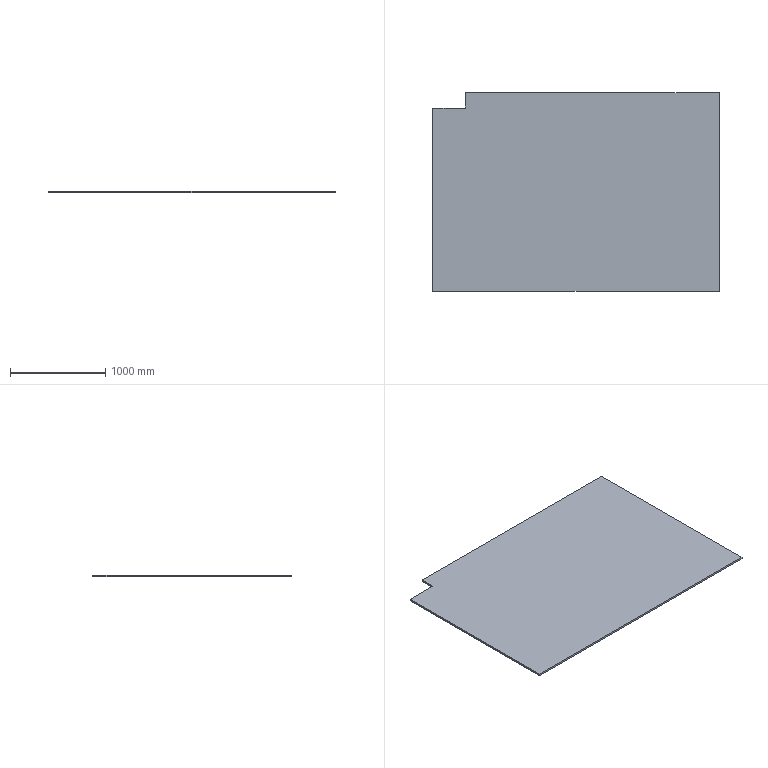Part | STEP file | 果蔬烘干机框架-103 | 1 solid | 8 faces | box 3000 x 2080 x 20 mm | volume 123712000 mm3 | plane 8
STEP:
#1=CARTESIAN_POINT('',(-1500.,880.,0.));
#2=VERTEX_POINT('',#1);
#3=CARTESIAN_POINT('',(-1500.,880.,20.));
#4=VERTEX_POINT('',#3);
#5=CARTESIAN_POINT('',(-1500.,880.,-80.));
#6=DIRECTION('',(0.,0.,1.));
#7=VECTOR('',#6,1000.);
#8=LINE('',#5,#7);
#9=EDGE_CURVE('',#2,#4,#8,.T.);
#10=ORIENTED_EDGE('',*,*,#9,.F.);
#11=CARTESIAN_POINT('',(-1500.,-1040.,0.));
#12=VERTEX_POINT('',#11);
#13=CARTESIAN_POINT('',(-1500.,1040.,0.));
#14=DIRECTION('',(0.,-1.,0.));
#15=VECTOR('',#14,1000.);
#16=LINE('',#13,#15);
#17=EDGE_CURVE('',#2,#12,#16,.T.);
#18=ORIENTED_EDGE('',*,*,#17,.T.);
#19=CARTESIAN_POINT('',(-1500.,-1040.,20.));
#20=VERTEX_POINT('',#19);
#21=CARTESIAN_POINT('',(-1500.,-1040.,20.));
#22=DIRECTION('',(0.,0.,-1.));
#23=VECTOR('',#22,1000.);
#24=LINE('',#21,#23);
#25=EDGE_CURVE('',#20,#12,#24,.T.);
#26=ORIENTED_EDGE('',*,*,#25,.F.);
#27=CARTESIAN_POINT('',(-1500.,1040.,20.));
#28=DIRECTION('',(0.,-1.,0.));
#29=VECTOR('',#28,1000.);
#30=LINE('',#27,#29);
#31=EDGE_CURVE('',#4,#20,#30,.T.);
#32=ORIENTED_EDGE('',*,*,#31,.F.);
#33=EDGE_LOOP('',(#10,#18,#26,#32));
#34=FACE_OUTER_BOUND('',#33,.T.);
#35=CARTESIAN_POINT('',(-1500.,1040.,20.));
#36=DIRECTION('',(1.,0.,0.));
#37=DIRECTION('',(0.,1.,0.));
#38=AXIS2_PLACEMENT_3D('',#35,#36,#37);
#39=PLANE('',#38);
#40=ADVANCED_FACE('',(#34),#39,.F.);
#41=CARTESIAN_POINT('',(1500.,-1040.,0.));
#42=VERTEX_POINT('',#41);
#43=CARTESIAN_POINT('',(1500.,1040.,0.));
#44=VERTEX_POINT('',#43);
#45=CARTESIAN_POINT('',(1500.,1040.,0.));
#46=DIRECTION('',(0.,1.,0.));
#47=VECTOR('',#46,1000.);
#48=LINE('',#45,#47);
#49=EDGE_CURVE('',#42,#44,#48,.T.);
#50=ORIENTED_EDGE('',*,*,#49,.T.);
#51=CARTESIAN_POINT('',(1500.,1040.,20.));
#52=VERTEX_POINT('',#51);
#53=CARTESIAN_POINT('',(1500.,1040.,20.));
#54=DIRECTION('',(0.,0.,-1.));
#55=VECTOR('',#54,1000.);
#56=LINE('',#53,#55);
#57=EDGE_CURVE('',#52,#44,#56,.T.);
#58=ORIENTED_EDGE('',*,*,#57,.F.);
#59=CARTESIAN_POINT('',(1500.,-1040.,20.));
#60=VERTEX_POINT('',#59);
#61=CARTESIAN_POINT('',(1500.,1040.,20.));
#62=DIRECTION('',(0.,1.,0.));
#63=VECTOR('',#62,1000.);
#64=LINE('',#61,#63);
#65=EDGE_CURVE('',#60,#52,#64,.T.);
#66=ORIENTED_EDGE('',*,*,#65,.F.);
#67=CARTESIAN_POINT('',(1500.,-1040.,20.));
#68=DIRECTION('',(0.,0.,-1.));
#69=VECTOR('',#68,1000.);
#70=LINE('',#67,#69);
#71=EDGE_CURVE('',#60,#42,#70,.T.);
#72=ORIENTED_EDGE('',*,*,#71,.T.);
#73=EDGE_LOOP('',(#50,#58,#66,#72));
#74=FACE_OUTER_BOUND('',#73,.T.);
#75=CARTESIAN_POINT('',(1500.,1040.,20.));
#76=DIRECTION('',(-1.,0.,0.));
#77=DIRECTION('',(0.,-1.,0.));
#78=AXIS2_PLACEMENT_3D('',#75,#76,#77);
#79=PLANE('',#78);
#80=ADVANCED_FACE('',(#74),#79,.F.);
#81=CARTESIAN_POINT('',(-1160.,1040.,0.));
#82=VERTEX_POINT('',#81);
#83=CARTESIAN_POINT('',(-1500.,1040.,0.));
#84=DIRECTION('',(-1.,0.,0.));
#85=VECTOR('',#84,1000.);
#86=LINE('',#83,#85);
#87=EDGE_CURVE('',#44,#82,#86,.T.);
#88=ORIENTED_EDGE('',*,*,#87,.T.);
#89=CARTESIAN_POINT('',(-1160.,1040.,20.));
#90=VERTEX_POINT('',#89);
#91=CARTESIAN_POINT('',(-1160.,1040.,-80.));
#92=DIRECTION('',(0.,0.,1.));
#93=VECTOR('',#92,1000.);
#94=LINE('',#91,#93);
#95=EDGE_CURVE('',#82,#90,#94,.T.);
#96=ORIENTED_EDGE('',*,*,#95,.T.);
#97=CARTESIAN_POINT('',(-1500.,1040.,20.));
#98=DIRECTION('',(-1.,0.,0.));
#99=VECTOR('',#98,1000.);
#100=LINE('',#97,#99);
#101=EDGE_CURVE('',#52,#90,#100,.T.);
#102=ORIENTED_EDGE('',*,*,#101,.F.);
#103=ORIENTED_EDGE('',*,*,#57,.T.);
#104=EDGE_LOOP('',(#88,#96,#102,#103));
#105=FACE_OUTER_BOUND('',#104,.T.);
#106=CARTESIAN_POINT('',(-1500.,1040.,20.));
#107=DIRECTION('',(0.,-1.,0.));
#108=DIRECTION('',(0.,0.,-1.));
#109=AXIS2_PLACEMENT_3D('',#106,#107,#108);
#110=PLANE('',#109);
#111=ADVANCED_FACE('',(#105),#110,.F.);
#112=CARTESIAN_POINT('',(-1500.,-1040.,0.));
#113=DIRECTION('',(1.,0.,0.));
#114=VECTOR('',#113,1000.);
#115=LINE('',#112,#114);
#116=EDGE_CURVE('',#12,#42,#115,.T.);
#117=ORIENTED_EDGE('',*,*,#116,.T.);
#118=ORIENTED_EDGE('',*,*,#71,.F.);
#119=CARTESIAN_POINT('',(-1500.,-1040.,20.));
#120=DIRECTION('',(1.,0.,0.));
#121=VECTOR('',#120,1000.);
#122=LINE('',#119,#121);
#123=EDGE_CURVE('',#20,#60,#122,.T.);
#124=ORIENTED_EDGE('',*,*,#123,.F.);
#125=ORIENTED_EDGE('',*,*,#25,.T.);
#126=EDGE_LOOP('',(#117,#118,#124,#125));
#127=FACE_OUTER_BOUND('',#126,.T.);
#128=CARTESIAN_POINT('',(-1500.,-1040.,20.));
#129=DIRECTION('',(0.,1.,0.));
#130=DIRECTION('',(0.,0.,1.));
#131=AXIS2_PLACEMENT_3D('',#128,#129,#130);
#132=PLANE('',#131);
#133=ADVANCED_FACE('',(#127),#132,.F.);
#134=CARTESIAN_POINT('',(-1160.,880.,20.));
#135=VERTEX_POINT('',#134);
#136=CARTESIAN_POINT('',(-1500.,880.,20.));
#137=DIRECTION('',(1.,0.,0.));
#138=VECTOR('',#137,1000.);
#139=LINE('',#136,#138);
#140=EDGE_CURVE('',#4,#135,#139,.T.);
#141=ORIENTED_EDGE('',*,*,#140,.F.);
#142=ORIENTED_EDGE('',*,*,#31,.T.);
#143=ORIENTED_EDGE('',*,*,#123,.T.);
#144=ORIENTED_EDGE('',*,*,#65,.T.);
#145=ORIENTED_EDGE('',*,*,#101,.T.);
#146=CARTESIAN_POINT('',(-1160.,1040.,20.));
#147=DIRECTION('',(0.,1.,0.));
#148=VECTOR('',#147,1000.);
#149=LINE('',#146,#148);
#150=EDGE_CURVE('',#135,#90,#149,.T.);
#151=ORIENTED_EDGE('',*,*,#150,.F.);
#152=EDGE_LOOP('',(#141,#142,#143,#144,#145,#151));
#153=FACE_OUTER_BOUND('',#152,.T.);
#154=CARTESIAN_POINT('',(0.,0.,20.));
#155=DIRECTION('',(0.,0.,1.));
#156=DIRECTION('',(1.,0.,0.));
#157=AXIS2_PLACEMENT_3D('',#154,#155,#156);
#158=PLANE('',#157);
#159=ADVANCED_FACE('',(#153),#158,.T.);
#160=CARTESIAN_POINT('',(-1160.,880.,0.));
#161=VERTEX_POINT('',#160);
#162=CARTESIAN_POINT('',(0.,880.,0.));
#163=DIRECTION('',(1.,0.,0.));
#164=VECTOR('',#163,1000.);
#165=LINE('',#162,#164);
#166=EDGE_CURVE('',#2,#161,#165,.T.);
#167=ORIENTED_EDGE('',*,*,#166,.T.);
#168=CARTESIAN_POINT('',(-1160.,0.,0.));
#169=DIRECTION('',(0.,1.,0.));
#170=VECTOR('',#169,1000.);
#171=LINE('',#168,#170);
#172=EDGE_CURVE('',#161,#82,#171,.T.);
#173=ORIENTED_EDGE('',*,*,#172,.T.);
#174=ORIENTED_EDGE('',*,*,#87,.F.);
#175=ORIENTED_EDGE('',*,*,#49,.F.);
#176=ORIENTED_EDGE('',*,*,#116,.F.);
#177=ORIENTED_EDGE('',*,*,#17,.F.);
#178=EDGE_LOOP('',(#167,#173,#174,#175,#176,#177));
#179=FACE_OUTER_BOUND('',#178,.T.);
#180=CARTESIAN_POINT('',(0.,0.,0.));
#181=DIRECTION('',(0.,0.,1.));
#182=DIRECTION('',(1.,0.,0.));
#183=AXIS2_PLACEMENT_3D('',#180,#181,#182);
#184=PLANE('',#183);
#185=ADVANCED_FACE('',(#179),#184,.F.);
#186=CARTESIAN_POINT('',(-1160.,880.,-80.));
#187=DIRECTION('',(0.,0.,1.));
#188=VECTOR('',#187,1000.);
#189=LINE('',#186,#188);
#190=EDGE_CURVE('',#161,#135,#189,.T.);
#191=ORIENTED_EDGE('',*,*,#190,.T.);
#192=ORIENTED_EDGE('',*,*,#150,.T.);
#193=ORIENTED_EDGE('',*,*,#95,.F.);
#194=ORIENTED_EDGE('',*,*,#172,.F.);
#195=EDGE_LOOP('',(#191,#192,#193,#194));
#196=FACE_OUTER_BOUND('',#195,.T.);
#197=CARTESIAN_POINT('',(-1160.,1040.,-80.));
#198=DIRECTION('',(1.,0.,0.));
#199=DIRECTION('',(0.,0.,-1.));
#200=AXIS2_PLACEMENT_3D('',#197,#198,#199);
#201=PLANE('',#200);
#202=ADVANCED_FACE('',(#196),#201,.F.);
#203=ORIENTED_EDGE('',*,*,#9,.T.);
#204=ORIENTED_EDGE('',*,*,#140,.T.);
#205=ORIENTED_EDGE('',*,*,#190,.F.);
#206=ORIENTED_EDGE('',*,*,#166,.F.);
#207=EDGE_LOOP('',(#203,#204,#205,#206));
#208=FACE_OUTER_BOUND('',#207,.T.);
#209=CARTESIAN_POINT('',(-1500.,880.,-80.));
#210=DIRECTION('',(0.,-1.,0.));
#211=DIRECTION('',(0.,0.,-1.));
#212=AXIS2_PLACEMENT_3D('',#209,#210,#211);
#213=PLANE('',#212);
#214=ADVANCED_FACE('',(#208),#213,.F.);
#215=CLOSED_SHELL('',(#40,#80,#111,#133,#159,#185,#202,#214));
#216=MANIFOLD_SOLID_BREP('',#215);
#217=CARTESIAN_POINT('',(0.,0.,0.));
#218=DIRECTION('',(0.,0.,1.));
#219=DIRECTION('',(1.,0.,0.));
#220=AXIS2_PLACEMENT_3D('',#217,#218,#219);
#221=(LENGTH_UNIT()NAMED_UNIT(*)SI_UNIT(.MILLI.,.METRE.));
#222=UNCERTAINTY_MEASURE_WITH_UNIT(LENGTH_MEASURE(0.00001),#221,'','');
#223=(NAMED_UNIT(*)PLANE_ANGLE_UNIT()SI_UNIT($,.RADIAN.));
#224=(NAMED_UNIT(*)SI_UNIT($,.STERADIAN.)SOLID_ANGLE_UNIT());
#225=(GEOMETRIC_REPRESENTATION_CONTEXT(3)GLOBAL_UNCERTAINTY_ASSIGNED_CONTEXT((#222))GLOBAL_UNIT_ASSIGNED_CONTEXT((#221,#223,#224))REPRESENTATION_CONTEXT('',''));
#226=ADVANCED_BREP_SHAPE_REPRESENTATION('',(#216,#220),#225);